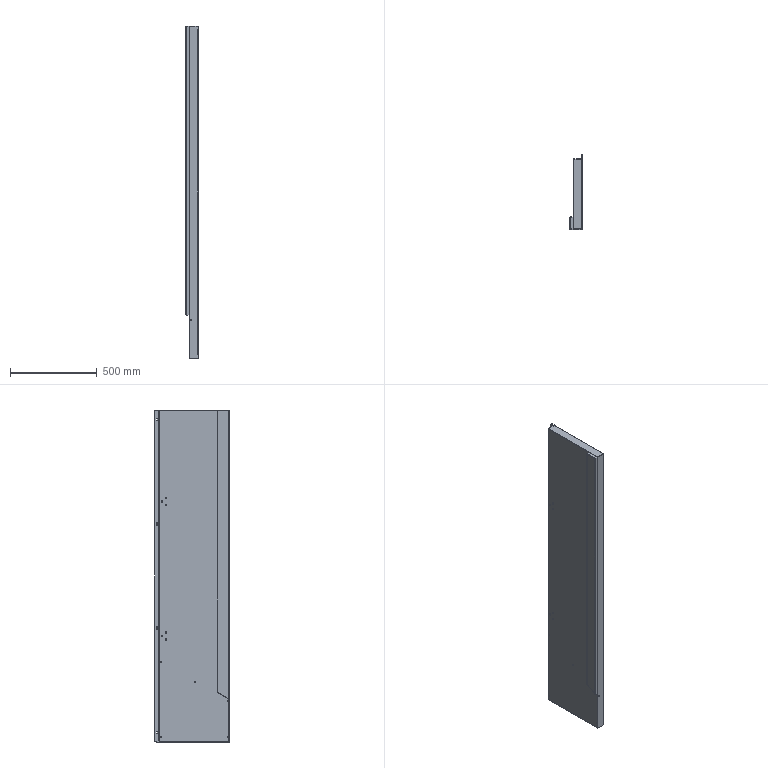Part | SolidWorks | 2 solids | 258 faces | box 70 x 430 x 1914 mm | volume 2035587 mm3 | plane 147 | cylinder 108 | spline 3 | commonest cylinder face diameters 6.4 x28 6 x16 7 x12 8.5 x12 2 x9 5 x9